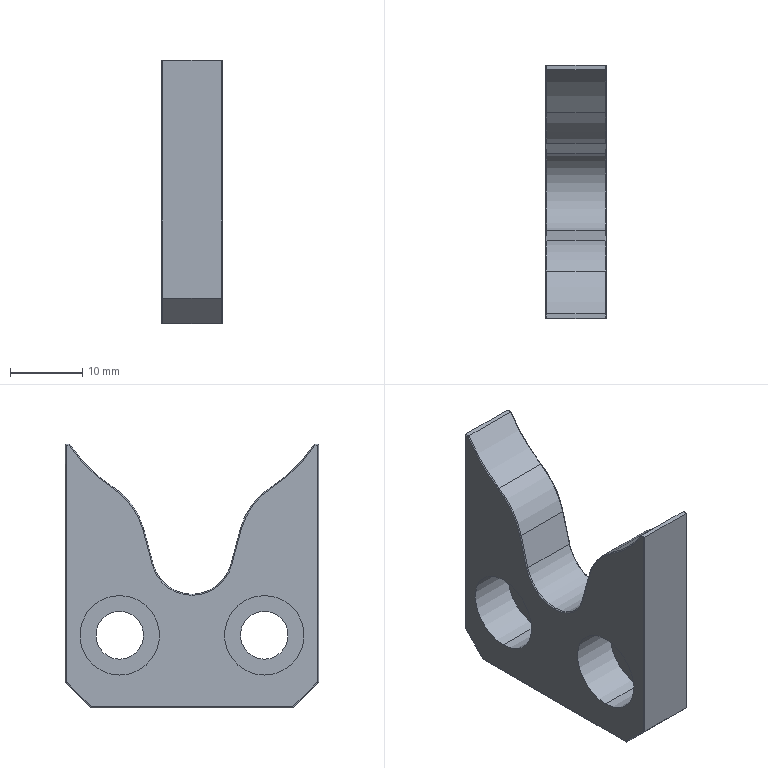Part | SolidWorks | features BaseBody 1 | 1 solid | 56 faces | box 8.4 x 35 x 36.4 mm | volume 6248 mm3 | cylinder 31 | plane 13 | spline 12 | commonest cylinder face diameters 0.28 x18 6.6 x4 11 x4 20.198 x2 40.396 x2 11.109 x1